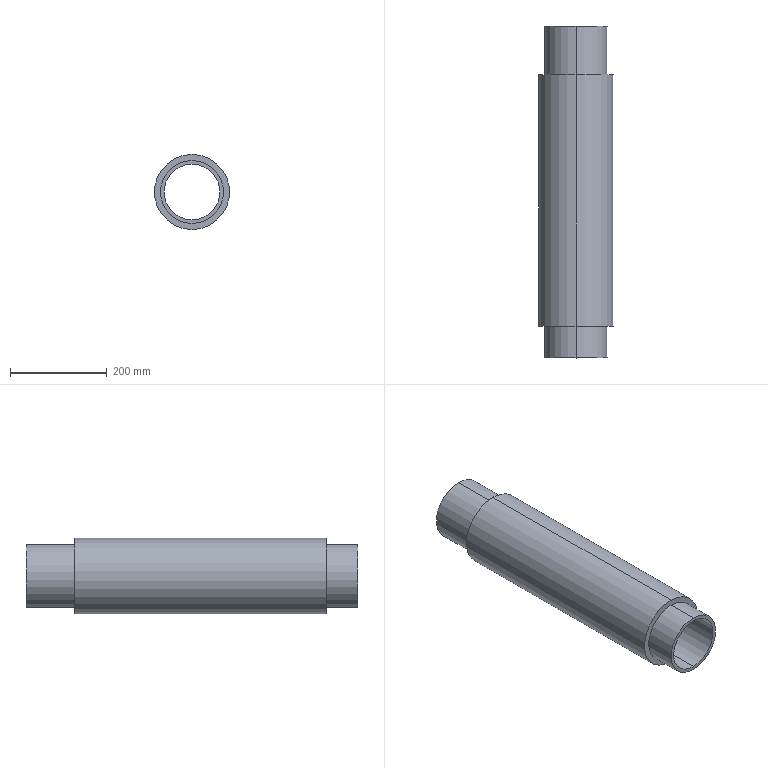Part | SolidWorks | features Revolution 1 | 1 solid | 12 faces | box 155 x 684.63 x 155 mm | volume 4883903 mm3 | cylinder 8 | plane 4 | commonest cylinder face diameters 130 x4 115 x2 155 x2
STEP:
#1=CARTESIAN_POINT('',(0.,370.012,65.));
#2=VERTEX_POINT('',#1);
#3=CARTESIAN_POINT('',(0.,370.012,-65.));
#4=VERTEX_POINT('',#3);
#5=CARTESIAN_POINT('',(0.,370.012,0.));
#6=DIRECTION('',(0.,1.,0.));
#7=DIRECTION('',(0.,0.,1.));
#8=AXIS2_PLACEMENT_3D('',#5,#6,#7);
#9=CIRCLE('',#8,65.);
#10=EDGE_CURVE('',#2,#4,#9,.T.);
#11=ORIENTED_EDGE('',*,*,#10,.T.);
#12=CARTESIAN_POINT('',(0.,470.012,-65.));
#13=VERTEX_POINT('',#12);
#14=CARTESIAN_POINT('',(0.,125.679,-65.));
#15=DIRECTION('',(0.,1.,0.));
#16=VECTOR('',#15,1000.);
#17=LINE('',#14,#16);
#18=EDGE_CURVE('',#4,#13,#17,.T.);
#19=ORIENTED_EDGE('',*,*,#18,.T.);
#20=CARTESIAN_POINT('',(0.,470.012,65.));
#21=VERTEX_POINT('',#20);
#22=CARTESIAN_POINT('',(0.,470.012,0.));
#23=DIRECTION('',(0.,1.,0.));
#24=DIRECTION('',(0.,0.,1.));
#25=AXIS2_PLACEMENT_3D('',#22,#23,#24);
#26=CIRCLE('',#25,65.);
#27=EDGE_CURVE('',#21,#13,#26,.T.);
#28=ORIENTED_EDGE('',*,*,#27,.F.);
#29=CARTESIAN_POINT('',(0.,125.679,65.));
#30=DIRECTION('',(0.,1.,0.));
#31=VECTOR('',#30,1000.);
#32=LINE('',#29,#31);
#33=EDGE_CURVE('',#2,#21,#32,.T.);
#34=ORIENTED_EDGE('',*,*,#33,.F.);
#35=EDGE_LOOP('',(#11,#19,#28,#34));
#36=FACE_OUTER_BOUND('',#35,.T.);
#37=CARTESIAN_POINT('',(0.,125.679,0.));
#38=DIRECTION('',(0.,1.,0.));
#39=DIRECTION('',(0.,0.,1.));
#40=AXIS2_PLACEMENT_3D('',#37,#38,#39);
#41=CYLINDRICAL_SURFACE('',#40,65.);
#42=ADVANCED_FACE('',(#36),#41,.T.);
#43=CARTESIAN_POINT('',(0.,-149.618,77.5));
#44=VERTEX_POINT('',#43);
#45=CARTESIAN_POINT('',(0.,-149.618,-77.5));
#46=VERTEX_POINT('',#45);
#47=CARTESIAN_POINT('',(0.,-149.618,0.));
#48=DIRECTION('',(0.,1.,0.));
#49=DIRECTION('',(0.,0.,1.));
#50=AXIS2_PLACEMENT_3D('',#47,#48,#49);
#51=CIRCLE('',#50,77.5);
#52=EDGE_CURVE('',#44,#46,#51,.T.);
#53=ORIENTED_EDGE('',*,*,#52,.T.);
#54=CARTESIAN_POINT('',(0.,370.012,-77.5));
#55=VERTEX_POINT('',#54);
#56=CARTESIAN_POINT('',(0.,125.679,-77.5));
#57=DIRECTION('',(0.,1.,0.));
#58=VECTOR('',#57,1000.);
#59=LINE('',#56,#58);
#60=EDGE_CURVE('',#46,#55,#59,.T.);
#61=ORIENTED_EDGE('',*,*,#60,.T.);
#62=CARTESIAN_POINT('',(0.,370.012,77.5));
#63=VERTEX_POINT('',#62);
#64=CARTESIAN_POINT('',(0.,370.012,0.));
#65=DIRECTION('',(0.,1.,0.));
#66=DIRECTION('',(0.,0.,1.));
#67=AXIS2_PLACEMENT_3D('',#64,#65,#66);
#68=CIRCLE('',#67,77.5);
#69=EDGE_CURVE('',#63,#55,#68,.T.);
#70=ORIENTED_EDGE('',*,*,#69,.F.);
#71=CARTESIAN_POINT('',(0.,125.679,77.5));
#72=DIRECTION('',(0.,1.,0.));
#73=VECTOR('',#72,1000.);
#74=LINE('',#71,#73);
#75=EDGE_CURVE('',#44,#63,#74,.T.);
#76=ORIENTED_EDGE('',*,*,#75,.F.);
#77=EDGE_LOOP('',(#53,#61,#70,#76));
#78=FACE_OUTER_BOUND('',#77,.T.);
#79=CARTESIAN_POINT('',(0.,125.679,0.));
#80=DIRECTION('',(0.,1.,0.));
#81=DIRECTION('',(0.,0.,1.));
#82=AXIS2_PLACEMENT_3D('',#79,#80,#81);
#83=CYLINDRICAL_SURFACE('',#82,77.5);
#84=ADVANCED_FACE('',(#78),#83,.T.);
#85=CARTESIAN_POINT('',(0.,-214.618,65.));
#86=VERTEX_POINT('',#85);
#87=CARTESIAN_POINT('',(0.,-214.618,-65.));
#88=VERTEX_POINT('',#87);
#89=CARTESIAN_POINT('',(0.,-214.618,0.));
#90=DIRECTION('',(0.,1.,0.));
#91=DIRECTION('',(0.,0.,1.));
#92=AXIS2_PLACEMENT_3D('',#89,#90,#91);
#93=CIRCLE('',#92,65.);
#94=EDGE_CURVE('',#86,#88,#93,.T.);
#95=ORIENTED_EDGE('',*,*,#94,.T.);
#96=CARTESIAN_POINT('',(0.,-149.618,-65.));
#97=VERTEX_POINT('',#96);
#98=CARTESIAN_POINT('',(0.,125.679,-65.));
#99=DIRECTION('',(0.,1.,0.));
#100=VECTOR('',#99,1000.);
#101=LINE('',#98,#100);
#102=EDGE_CURVE('',#88,#97,#101,.T.);
#103=ORIENTED_EDGE('',*,*,#102,.T.);
#104=CARTESIAN_POINT('',(0.,-149.618,65.));
#105=VERTEX_POINT('',#104);
#106=CARTESIAN_POINT('',(0.,-149.618,0.));
#107=DIRECTION('',(0.,1.,0.));
#108=DIRECTION('',(0.,0.,1.));
#109=AXIS2_PLACEMENT_3D('',#106,#107,#108);
#110=CIRCLE('',#109,65.);
#111=EDGE_CURVE('',#105,#97,#110,.T.);
#112=ORIENTED_EDGE('',*,*,#111,.F.);
#113=CARTESIAN_POINT('',(0.,125.679,65.));
#114=DIRECTION('',(0.,1.,0.));
#115=VECTOR('',#114,1000.);
#116=LINE('',#113,#115);
#117=EDGE_CURVE('',#86,#105,#116,.T.);
#118=ORIENTED_EDGE('',*,*,#117,.F.);
#119=EDGE_LOOP('',(#95,#103,#112,#118));
#120=FACE_OUTER_BOUND('',#119,.T.);
#121=CARTESIAN_POINT('',(0.,125.679,0.));
#122=DIRECTION('',(0.,1.,0.));
#123=DIRECTION('',(0.,0.,1.));
#124=AXIS2_PLACEMENT_3D('',#121,#122,#123);
#125=CYLINDRICAL_SURFACE('',#124,65.);
#126=ADVANCED_FACE('',(#120),#125,.T.);
#127=CARTESIAN_POINT('',(0.,-214.618,-57.5));
#128=VERTEX_POINT('',#127);
#129=CARTESIAN_POINT('',(0.,-214.618,57.5));
#130=VERTEX_POINT('',#129);
#131=CARTESIAN_POINT('',(0.,-214.618,0.));
#132=DIRECTION('',(0.,1.,0.));
#133=DIRECTION('',(0.,0.,1.));
#134=AXIS2_PLACEMENT_3D('',#131,#132,#133);
#135=CIRCLE('',#134,57.5);
#136=EDGE_CURVE('',#128,#130,#135,.T.);
#137=ORIENTED_EDGE('',*,*,#136,.F.);
#138=CARTESIAN_POINT('',(0.,470.012,-57.5));
#139=VERTEX_POINT('',#138);
#140=CARTESIAN_POINT('',(0.,125.679,-57.5));
#141=DIRECTION('',(0.,1.,0.));
#142=VECTOR('',#141,1000.);
#143=LINE('',#140,#142);
#144=EDGE_CURVE('',#128,#139,#143,.T.);
#145=ORIENTED_EDGE('',*,*,#144,.T.);
#146=CARTESIAN_POINT('',(0.,470.012,57.5));
#147=VERTEX_POINT('',#146);
#148=CARTESIAN_POINT('',(0.,470.012,0.));
#149=DIRECTION('',(0.,1.,0.));
#150=DIRECTION('',(0.,0.,1.));
#151=AXIS2_PLACEMENT_3D('',#148,#149,#150);
#152=CIRCLE('',#151,57.5);
#153=EDGE_CURVE('',#139,#147,#152,.T.);
#154=ORIENTED_EDGE('',*,*,#153,.T.);
#155=CARTESIAN_POINT('',(0.,125.679,57.5));
#156=DIRECTION('',(0.,1.,0.));
#157=VECTOR('',#156,1000.);
#158=LINE('',#155,#157);
#159=EDGE_CURVE('',#130,#147,#158,.T.);
#160=ORIENTED_EDGE('',*,*,#159,.F.);
#161=EDGE_LOOP('',(#137,#145,#154,#160));
#162=FACE_OUTER_BOUND('',#161,.T.);
#163=CARTESIAN_POINT('',(0.,125.679,0.));
#164=DIRECTION('',(0.,1.,0.));
#165=DIRECTION('',(0.,0.,1.));
#166=AXIS2_PLACEMENT_3D('',#163,#164,#165);
#167=CYLINDRICAL_SURFACE('',#166,57.5);
#168=ADVANCED_FACE('',(#162),#167,.F.);
#169=CARTESIAN_POINT('',(0.,470.012,0.));
#170=DIRECTION('',(0.,1.,0.));
#171=DIRECTION('',(0.,0.,1.));
#172=AXIS2_PLACEMENT_3D('',#169,#170,#171);
#173=CIRCLE('',#172,57.5);
#174=EDGE_CURVE('',#147,#139,#173,.T.);
#175=ORIENTED_EDGE('',*,*,#174,.F.);
#176=ORIENTED_EDGE('',*,*,#153,.F.);
#177=EDGE_LOOP('',(#175,#176));
#178=FACE_BOUND('',#177,.T.);
#179=ORIENTED_EDGE('',*,*,#27,.T.);
#180=CARTESIAN_POINT('',(0.,470.012,0.));
#181=DIRECTION('',(0.,1.,0.));
#182=DIRECTION('',(0.,0.,1.));
#183=AXIS2_PLACEMENT_3D('',#180,#181,#182);
#184=CIRCLE('',#183,65.);
#185=EDGE_CURVE('',#13,#21,#184,.T.);
#186=ORIENTED_EDGE('',*,*,#185,.T.);
#187=EDGE_LOOP('',(#179,#186));
#188=FACE_OUTER_BOUND('',#187,.T.);
#189=CARTESIAN_POINT('',(65.,470.012,0.));
#190=DIRECTION('',(0.,-1.,0.));
#191=DIRECTION('',(0.,0.,-1.));
#192=AXIS2_PLACEMENT_3D('',#189,#190,#191);
#193=PLANE('',#192);
#194=ADVANCED_FACE('',(#178,#188),#193,.F.);
#195=ORIENTED_EDGE('',*,*,#144,.F.);
#196=CARTESIAN_POINT('',(0.,-214.618,0.));
#197=DIRECTION('',(0.,1.,0.));
#198=DIRECTION('',(0.,0.,1.));
#199=AXIS2_PLACEMENT_3D('',#196,#197,#198);
#200=CIRCLE('',#199,57.5);
#201=EDGE_CURVE('',#130,#128,#200,.T.);
#202=ORIENTED_EDGE('',*,*,#201,.F.);
#203=ORIENTED_EDGE('',*,*,#159,.T.);
#204=ORIENTED_EDGE('',*,*,#174,.T.);
#205=EDGE_LOOP('',(#195,#202,#203,#204));
#206=FACE_OUTER_BOUND('',#205,.T.);
#207=CARTESIAN_POINT('',(0.,125.679,0.));
#208=DIRECTION('',(0.,1.,0.));
#209=DIRECTION('',(0.,0.,1.));
#210=AXIS2_PLACEMENT_3D('',#207,#208,#209);
#211=CYLINDRICAL_SURFACE('',#210,57.5);
#212=ADVANCED_FACE('',(#206),#211,.F.);
#213=ORIENTED_EDGE('',*,*,#94,.F.);
#214=CARTESIAN_POINT('',(0.,-214.618,0.));
#215=DIRECTION('',(0.,1.,0.));
#216=DIRECTION('',(0.,0.,1.));
#217=AXIS2_PLACEMENT_3D('',#214,#215,#216);
#218=CIRCLE('',#217,65.);
#219=EDGE_CURVE('',#88,#86,#218,.T.);
#220=ORIENTED_EDGE('',*,*,#219,.F.);
#221=EDGE_LOOP('',(#213,#220));
#222=FACE_OUTER_BOUND('',#221,.T.);
#223=ORIENTED_EDGE('',*,*,#201,.T.);
#224=ORIENTED_EDGE('',*,*,#136,.T.);
#225=EDGE_LOOP('',(#223,#224));
#226=FACE_BOUND('',#225,.T.);
#227=CARTESIAN_POINT('',(57.5,-214.618,0.));
#228=DIRECTION('',(0.,1.,0.));
#229=DIRECTION('',(0.,0.,1.));
#230=AXIS2_PLACEMENT_3D('',#227,#228,#229);
#231=PLANE('',#230);
#232=ADVANCED_FACE('',(#222,#226),#231,.F.);
#233=ORIENTED_EDGE('',*,*,#102,.F.);
#234=ORIENTED_EDGE('',*,*,#219,.T.);
#235=ORIENTED_EDGE('',*,*,#117,.T.);
#236=CARTESIAN_POINT('',(0.,-149.618,0.));
#237=DIRECTION('',(0.,1.,0.));
#238=DIRECTION('',(0.,0.,1.));
#239=AXIS2_PLACEMENT_3D('',#236,#237,#238);
#240=CIRCLE('',#239,65.);
#241=EDGE_CURVE('',#97,#105,#240,.T.);
#242=ORIENTED_EDGE('',*,*,#241,.F.);
#243=EDGE_LOOP('',(#233,#234,#235,#242));
#244=FACE_OUTER_BOUND('',#243,.T.);
#245=CARTESIAN_POINT('',(0.,125.679,0.));
#246=DIRECTION('',(0.,1.,0.));
#247=DIRECTION('',(0.,0.,1.));
#248=AXIS2_PLACEMENT_3D('',#245,#246,#247);
#249=CYLINDRICAL_SURFACE('',#248,65.);
#250=ADVANCED_FACE('',(#244),#249,.T.);
#251=ORIENTED_EDGE('',*,*,#52,.F.);
#252=CARTESIAN_POINT('',(0.,-149.618,0.));
#253=DIRECTION('',(0.,1.,0.));
#254=DIRECTION('',(0.,0.,1.));
#255=AXIS2_PLACEMENT_3D('',#252,#253,#254);
#256=CIRCLE('',#255,77.5);
#257=EDGE_CURVE('',#46,#44,#256,.T.);
#258=ORIENTED_EDGE('',*,*,#257,.F.);
#259=EDGE_LOOP('',(#251,#258));
#260=FACE_OUTER_BOUND('',#259,.T.);
#261=ORIENTED_EDGE('',*,*,#111,.T.);
#262=ORIENTED_EDGE('',*,*,#241,.T.);
#263=EDGE_LOOP('',(#261,#262));
#264=FACE_BOUND('',#263,.T.);
#265=CARTESIAN_POINT('',(65.,-149.618,0.));
#266=DIRECTION('',(0.,1.,0.));
#267=DIRECTION('',(0.,0.,1.));
#268=AXIS2_PLACEMENT_3D('',#265,#266,#267);
#269=PLANE('',#268);
#270=ADVANCED_FACE('',(#260,#264),#269,.F.);
#271=ORIENTED_EDGE('',*,*,#60,.F.);
#272=ORIENTED_EDGE('',*,*,#257,.T.);
#273=ORIENTED_EDGE('',*,*,#75,.T.);
#274=CARTESIAN_POINT('',(0.,370.012,0.));
#275=DIRECTION('',(0.,1.,0.));
#276=DIRECTION('',(0.,0.,1.));
#277=AXIS2_PLACEMENT_3D('',#274,#275,#276);
#278=CIRCLE('',#277,77.5);
#279=EDGE_CURVE('',#55,#63,#278,.T.);
#280=ORIENTED_EDGE('',*,*,#279,.F.);
#281=EDGE_LOOP('',(#271,#272,#273,#280));
#282=FACE_OUTER_BOUND('',#281,.T.);
#283=CARTESIAN_POINT('',(0.,125.679,0.));
#284=DIRECTION('',(0.,1.,0.));
#285=DIRECTION('',(0.,0.,1.));
#286=AXIS2_PLACEMENT_3D('',#283,#284,#285);
#287=CYLINDRICAL_SURFACE('',#286,77.5);
#288=ADVANCED_FACE('',(#282),#287,.T.);
#289=ORIENTED_EDGE('',*,*,#10,.F.);
#290=CARTESIAN_POINT('',(0.,370.012,0.));
#291=DIRECTION('',(0.,1.,0.));
#292=DIRECTION('',(0.,0.,1.));
#293=AXIS2_PLACEMENT_3D('',#290,#291,#292);
#294=CIRCLE('',#293,65.);
#295=EDGE_CURVE('',#4,#2,#294,.T.);
#296=ORIENTED_EDGE('',*,*,#295,.F.);
#297=EDGE_LOOP('',(#289,#296));
#298=FACE_BOUND('',#297,.T.);
#299=ORIENTED_EDGE('',*,*,#69,.T.);
#300=ORIENTED_EDGE('',*,*,#279,.T.);
#301=EDGE_LOOP('',(#299,#300));
#302=FACE_OUTER_BOUND('',#301,.T.);
#303=CARTESIAN_POINT('',(77.5,370.012,0.));
#304=DIRECTION('',(0.,-1.,0.));
#305=DIRECTION('',(0.,0.,-1.));
#306=AXIS2_PLACEMENT_3D('',#303,#304,#305);
#307=PLANE('',#306);
#308=ADVANCED_FACE('',(#298,#302),#307,.F.);
#309=ORIENTED_EDGE('',*,*,#18,.F.);
#310=ORIENTED_EDGE('',*,*,#295,.T.);
#311=ORIENTED_EDGE('',*,*,#33,.T.);
#312=ORIENTED_EDGE('',*,*,#185,.F.);
#313=EDGE_LOOP('',(#309,#310,#311,#312));
#314=FACE_OUTER_BOUND('',#313,.T.);
#315=CARTESIAN_POINT('',(0.,125.679,0.));
#316=DIRECTION('',(0.,1.,0.));
#317=DIRECTION('',(0.,0.,1.));
#318=AXIS2_PLACEMENT_3D('',#315,#316,#317);
#319=CYLINDRICAL_SURFACE('',#318,65.);
#320=ADVANCED_FACE('',(#314),#319,.T.);
#321=CLOSED_SHELL('',(#42,#84,#126,#168,#194,#212,#232,#250,#270,#288,#308,#320));
#322=MANIFOLD_SOLID_BREP('',#321);
#323=CARTESIAN_POINT('',(0.,0.,0.));
#324=DIRECTION('',(0.,0.,1.));
#325=DIRECTION('',(1.,0.,0.));
#326=AXIS2_PLACEMENT_3D('',#323,#324,#325);
#327=(LENGTH_UNIT()NAMED_UNIT(*)SI_UNIT(.MILLI.,.METRE.));
#328=UNCERTAINTY_MEASURE_WITH_UNIT(LENGTH_MEASURE(0.00001),#327,'','');
#329=(NAMED_UNIT(*)PLANE_ANGLE_UNIT()SI_UNIT($,.RADIAN.));
#330=(NAMED_UNIT(*)SI_UNIT($,.STERADIAN.)SOLID_ANGLE_UNIT());
#331=(GEOMETRIC_REPRESENTATION_CONTEXT(3)GLOBAL_UNCERTAINTY_ASSIGNED_CONTEXT((#328))GLOBAL_UNIT_ASSIGNED_CONTEXT((#327,#329,#330))REPRESENTATION_CONTEXT('',''));
#332=ADVANCED_BREP_SHAPE_REPRESENTATION('',(#322,#326),#331);